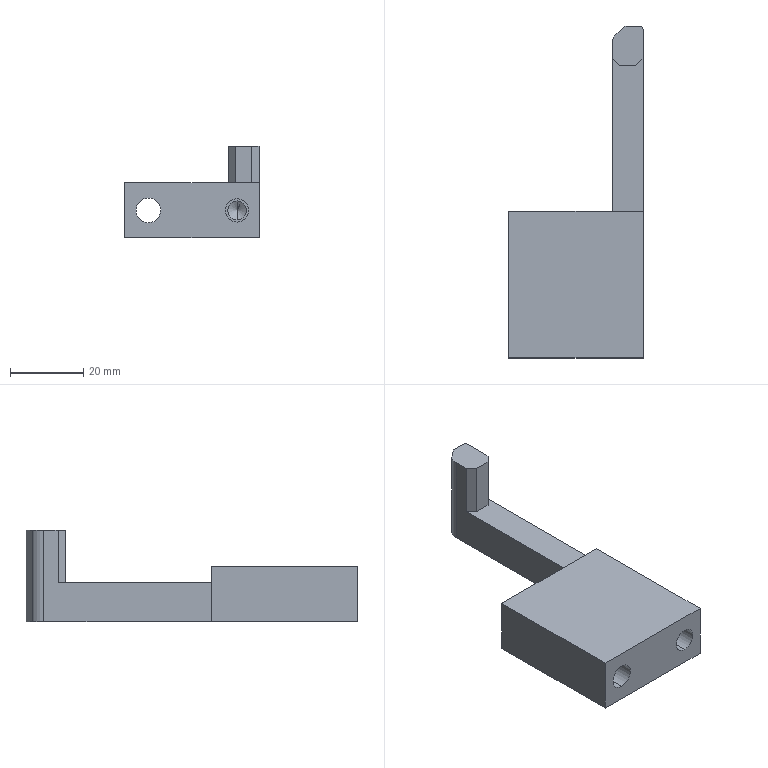Part | STEP file | 1_id1002_x_t | 1 solid | 25 faces | box 36.508 x 90.344 x 25 mm | volume 24887 mm3 | plane 15 | cylinder 8 | cone 2 | commonest cylinder face diameters 5.105 x2 6.35 x2 6.731 x2 2 x1 8 x1